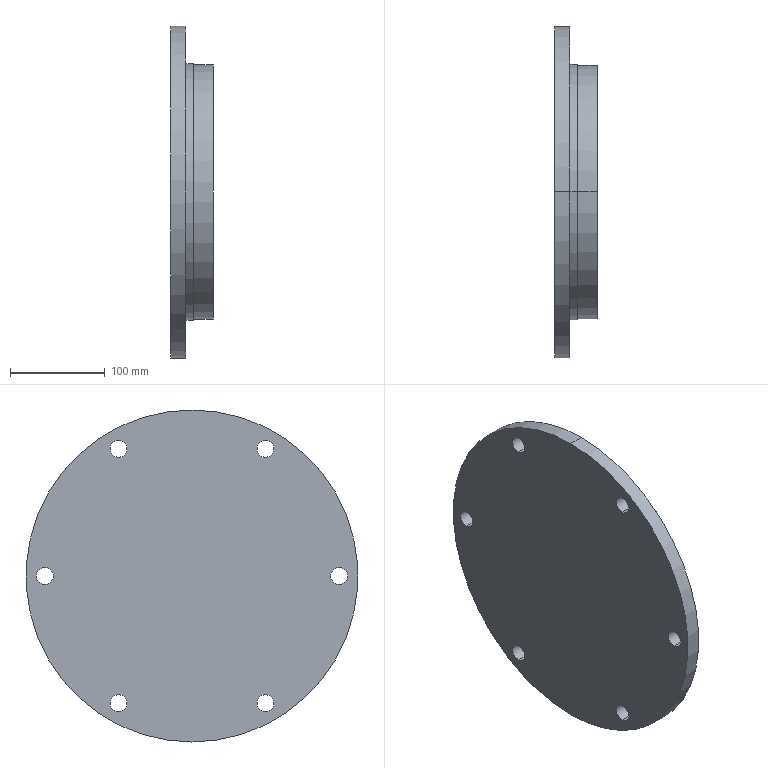Part | NX | features BREP 1 | 1 solid | 27 faces | box 45 x 350 x 350 mm | volume 1642719 mm3 | cylinder 18 | plane 5 | torus 2 | cone 2 | commonest cylinder face diameters 18 x12 268 x2 270 x2 350 x2
STEP:
#1=CARTESIAN_POINT('',(16.,77.5,-143.234));
#2=VERTEX_POINT('',#1);
#3=CARTESIAN_POINT('',(16.,77.5,-125.234));
#4=VERTEX_POINT('',#3);
#5=CARTESIAN_POINT('',(16.,77.5,-134.234));
#6=DIRECTION('',(-1.,0.,0.));
#7=DIRECTION('',(0.,0.,1.));
#8=AXIS2_PLACEMENT_3D('',#5,#6,#7);
#9=CIRCLE('',#8,9.);
#10=EDGE_CURVE('',#2,#4,#9,.T.);
#11=ORIENTED_EDGE('',*,*,#10,.F.);
#12=CARTESIAN_POINT('',(0.,77.5,-143.234));
#13=VERTEX_POINT('',#12);
#14=CARTESIAN_POINT('',(45.,77.5,-143.234));
#15=DIRECTION('',(-1.,0.,0.));
#16=VECTOR('',#15,1000.);
#17=LINE('',#14,#16);
#18=EDGE_CURVE('',#2,#13,#17,.T.);
#19=ORIENTED_EDGE('',*,*,#18,.T.);
#20=CARTESIAN_POINT('',(0.,77.5,-125.234));
#21=VERTEX_POINT('',#20);
#22=CARTESIAN_POINT('',(0.,77.5,-134.234));
#23=DIRECTION('',(-1.,0.,0.));
#24=DIRECTION('',(0.,0.866,0.5));
#25=AXIS2_PLACEMENT_3D('',#22,#23,#24);
#26=CIRCLE('',#25,9.);
#27=EDGE_CURVE('',#13,#21,#26,.T.);
#28=ORIENTED_EDGE('',*,*,#27,.T.);
#29=CARTESIAN_POINT('',(45.,77.5,-125.234));
#30=DIRECTION('',(-1.,0.,0.));
#31=VECTOR('',#30,1000.);
#32=LINE('',#29,#31);
#33=EDGE_CURVE('',#4,#21,#32,.T.);
#34=ORIENTED_EDGE('',*,*,#33,.F.);
#35=EDGE_LOOP('',(#11,#19,#28,#34));
#36=FACE_BOUND('',#35,.T.);
#37=CARTESIAN_POINT('',(45.,77.5,-134.234));
#38=DIRECTION('',(-1.,0.,0.));
#39=DIRECTION('',(0.,0.,-1.));
#40=AXIS2_PLACEMENT_3D('',#37,#38,#39);
#41=CYLINDRICAL_SURFACE('',#40,9.);
#42=ADVANCED_FACE('',(#36),#41,.F.);
#43=CARTESIAN_POINT('',(16.,-77.5,-143.234));
#44=VERTEX_POINT('',#43);
#45=CARTESIAN_POINT('',(16.,-77.5,-125.234));
#46=VERTEX_POINT('',#45);
#47=CARTESIAN_POINT('',(16.,-77.5,-134.234));
#48=DIRECTION('',(-1.,0.,0.));
#49=DIRECTION('',(0.,0.,1.));
#50=AXIS2_PLACEMENT_3D('',#47,#48,#49);
#51=CIRCLE('',#50,9.);
#52=EDGE_CURVE('',#44,#46,#51,.T.);
#53=ORIENTED_EDGE('',*,*,#52,.F.);
#54=CARTESIAN_POINT('',(0.,-77.5,-143.234));
#55=VERTEX_POINT('',#54);
#56=CARTESIAN_POINT('',(45.,-77.5,-143.234));
#57=DIRECTION('',(-1.,0.,0.));
#58=VECTOR('',#57,1000.);
#59=LINE('',#56,#58);
#60=EDGE_CURVE('',#44,#55,#59,.T.);
#61=ORIENTED_EDGE('',*,*,#60,.T.);
#62=CARTESIAN_POINT('',(0.,-77.5,-125.234));
#63=VERTEX_POINT('',#62);
#64=CARTESIAN_POINT('',(0.,-77.5,-134.234));
#65=DIRECTION('',(-1.,0.,0.));
#66=DIRECTION('',(0.,0.866,-0.5));
#67=AXIS2_PLACEMENT_3D('',#64,#65,#66);
#68=CIRCLE('',#67,9.);
#69=EDGE_CURVE('',#55,#63,#68,.T.);
#70=ORIENTED_EDGE('',*,*,#69,.T.);
#71=CARTESIAN_POINT('',(45.,-77.5,-125.234));
#72=DIRECTION('',(-1.,0.,0.));
#73=VECTOR('',#72,1000.);
#74=LINE('',#71,#73);
#75=EDGE_CURVE('',#46,#63,#74,.T.);
#76=ORIENTED_EDGE('',*,*,#75,.F.);
#77=EDGE_LOOP('',(#53,#61,#70,#76));
#78=FACE_BOUND('',#77,.T.);
#79=CARTESIAN_POINT('',(45.,-77.5,-134.234));
#80=DIRECTION('',(-1.,0.,0.));
#81=DIRECTION('',(0.,0.,-1.));
#82=AXIS2_PLACEMENT_3D('',#79,#80,#81);
#83=CYLINDRICAL_SURFACE('',#82,9.);
#84=ADVANCED_FACE('',(#78),#83,.F.);
#85=CARTESIAN_POINT('',(16.,-155.,-9.));
#86=VERTEX_POINT('',#85);
#87=CARTESIAN_POINT('',(16.,-155.,9.));
#88=VERTEX_POINT('',#87);
#89=CARTESIAN_POINT('',(16.,-155.,0.));
#90=DIRECTION('',(-1.,0.,0.));
#91=DIRECTION('',(0.,0.,1.));
#92=AXIS2_PLACEMENT_3D('',#89,#90,#91);
#93=CIRCLE('',#92,9.);
#94=EDGE_CURVE('',#86,#88,#93,.T.);
#95=ORIENTED_EDGE('',*,*,#94,.F.);
#96=CARTESIAN_POINT('',(0.,-155.,-9.));
#97=VERTEX_POINT('',#96);
#98=CARTESIAN_POINT('',(45.,-155.,-9.));
#99=DIRECTION('',(-1.,0.,0.));
#100=VECTOR('',#99,1000.);
#101=LINE('',#98,#100);
#102=EDGE_CURVE('',#86,#97,#101,.T.);
#103=ORIENTED_EDGE('',*,*,#102,.T.);
#104=CARTESIAN_POINT('',(0.,-155.,9.));
#105=VERTEX_POINT('',#104);
#106=CARTESIAN_POINT('',(0.,-155.,0.));
#107=DIRECTION('',(-1.,0.,0.));
#108=DIRECTION('',(0.,0.,-1.));
#109=AXIS2_PLACEMENT_3D('',#106,#107,#108);
#110=CIRCLE('',#109,9.);
#111=EDGE_CURVE('',#97,#105,#110,.T.);
#112=ORIENTED_EDGE('',*,*,#111,.T.);
#113=CARTESIAN_POINT('',(45.,-155.,9.));
#114=DIRECTION('',(-1.,0.,0.));
#115=VECTOR('',#114,1000.);
#116=LINE('',#113,#115);
#117=EDGE_CURVE('',#88,#105,#116,.T.);
#118=ORIENTED_EDGE('',*,*,#117,.F.);
#119=EDGE_LOOP('',(#95,#103,#112,#118));
#120=FACE_BOUND('',#119,.T.);
#121=CARTESIAN_POINT('',(45.,-155.,0.));
#122=DIRECTION('',(-1.,0.,0.));
#123=DIRECTION('',(0.,0.,-1.));
#124=AXIS2_PLACEMENT_3D('',#121,#122,#123);
#125=CYLINDRICAL_SURFACE('',#124,9.);
#126=ADVANCED_FACE('',(#120),#125,.F.);
#127=CARTESIAN_POINT('',(16.,-77.5,125.234));
#128=VERTEX_POINT('',#127);
#129=CARTESIAN_POINT('',(16.,-77.5,143.234));
#130=VERTEX_POINT('',#129);
#131=CARTESIAN_POINT('',(16.,-77.5,134.234));
#132=DIRECTION('',(-1.,0.,0.));
#133=DIRECTION('',(0.,0.,1.));
#134=AXIS2_PLACEMENT_3D('',#131,#132,#133);
#135=CIRCLE('',#134,9.);
#136=EDGE_CURVE('',#128,#130,#135,.T.);
#137=ORIENTED_EDGE('',*,*,#136,.F.);
#138=CARTESIAN_POINT('',(0.,-77.5,125.234));
#139=VERTEX_POINT('',#138);
#140=CARTESIAN_POINT('',(45.,-77.5,125.234));
#141=DIRECTION('',(-1.,0.,0.));
#142=VECTOR('',#141,1000.);
#143=LINE('',#140,#142);
#144=EDGE_CURVE('',#128,#139,#143,.T.);
#145=ORIENTED_EDGE('',*,*,#144,.T.);
#146=CARTESIAN_POINT('',(0.,-77.5,143.234));
#147=VERTEX_POINT('',#146);
#148=CARTESIAN_POINT('',(0.,-77.5,134.234));
#149=DIRECTION('',(-1.,0.,0.));
#150=DIRECTION('',(0.,-0.866,-0.5));
#151=AXIS2_PLACEMENT_3D('',#148,#149,#150);
#152=CIRCLE('',#151,9.);
#153=EDGE_CURVE('',#139,#147,#152,.T.);
#154=ORIENTED_EDGE('',*,*,#153,.T.);
#155=CARTESIAN_POINT('',(45.,-77.5,143.234));
#156=DIRECTION('',(-1.,0.,0.));
#157=VECTOR('',#156,1000.);
#158=LINE('',#155,#157);
#159=EDGE_CURVE('',#130,#147,#158,.T.);
#160=ORIENTED_EDGE('',*,*,#159,.F.);
#161=EDGE_LOOP('',(#137,#145,#154,#160));
#162=FACE_BOUND('',#161,.T.);
#163=CARTESIAN_POINT('',(45.,-77.5,134.234));
#164=DIRECTION('',(-1.,0.,0.));
#165=DIRECTION('',(0.,0.,-1.));
#166=AXIS2_PLACEMENT_3D('',#163,#164,#165);
#167=CYLINDRICAL_SURFACE('',#166,9.);
#168=ADVANCED_FACE('',(#162),#167,.F.);
#169=CARTESIAN_POINT('',(16.,77.5,125.234));
#170=VERTEX_POINT('',#169);
#171=CARTESIAN_POINT('',(16.,77.5,143.234));
#172=VERTEX_POINT('',#171);
#173=CARTESIAN_POINT('',(16.,77.5,134.234));
#174=DIRECTION('',(-1.,0.,0.));
#175=DIRECTION('',(0.,0.,1.));
#176=AXIS2_PLACEMENT_3D('',#173,#174,#175);
#177=CIRCLE('',#176,9.);
#178=EDGE_CURVE('',#170,#172,#177,.T.);
#179=ORIENTED_EDGE('',*,*,#178,.F.);
#180=CARTESIAN_POINT('',(0.,77.5,125.234));
#181=VERTEX_POINT('',#180);
#182=CARTESIAN_POINT('',(45.,77.5,125.234));
#183=DIRECTION('',(-1.,0.,0.));
#184=VECTOR('',#183,1000.);
#185=LINE('',#182,#184);
#186=EDGE_CURVE('',#170,#181,#185,.T.);
#187=ORIENTED_EDGE('',*,*,#186,.T.);
#188=CARTESIAN_POINT('',(0.,77.5,143.234));
#189=VERTEX_POINT('',#188);
#190=CARTESIAN_POINT('',(0.,77.5,134.234));
#191=DIRECTION('',(-1.,0.,0.));
#192=DIRECTION('',(0.,-0.866,0.5));
#193=AXIS2_PLACEMENT_3D('',#190,#191,#192);
#194=CIRCLE('',#193,9.);
#195=EDGE_CURVE('',#181,#189,#194,.T.);
#196=ORIENTED_EDGE('',*,*,#195,.T.);
#197=CARTESIAN_POINT('',(45.,77.5,143.234));
#198=DIRECTION('',(-1.,0.,0.));
#199=VECTOR('',#198,1000.);
#200=LINE('',#197,#199);
#201=EDGE_CURVE('',#172,#189,#200,.T.);
#202=ORIENTED_EDGE('',*,*,#201,.F.);
#203=EDGE_LOOP('',(#179,#187,#196,#202));
#204=FACE_BOUND('',#203,.T.);
#205=CARTESIAN_POINT('',(45.,77.5,134.234));
#206=DIRECTION('',(-1.,0.,0.));
#207=DIRECTION('',(0.,0.,-1.));
#208=AXIS2_PLACEMENT_3D('',#205,#206,#207);
#209=CYLINDRICAL_SURFACE('',#208,9.);
#210=ADVANCED_FACE('',(#204),#209,.F.);
#211=CARTESIAN_POINT('',(16.,155.,-9.));
#212=VERTEX_POINT('',#211);
#213=CARTESIAN_POINT('',(16.,155.,9.));
#214=VERTEX_POINT('',#213);
#215=CARTESIAN_POINT('',(16.,155.,0.));
#216=DIRECTION('',(-1.,0.,0.));
#217=DIRECTION('',(0.,0.,1.));
#218=AXIS2_PLACEMENT_3D('',#215,#216,#217);
#219=CIRCLE('',#218,9.);
#220=EDGE_CURVE('',#212,#214,#219,.T.);
#221=ORIENTED_EDGE('',*,*,#220,.F.);
#222=CARTESIAN_POINT('',(0.,155.,-9.));
#223=VERTEX_POINT('',#222);
#224=CARTESIAN_POINT('',(45.,155.,-9.));
#225=DIRECTION('',(-1.,0.,0.));
#226=VECTOR('',#225,1000.);
#227=LINE('',#224,#226);
#228=EDGE_CURVE('',#212,#223,#227,.T.);
#229=ORIENTED_EDGE('',*,*,#228,.T.);
#230=CARTESIAN_POINT('',(0.,155.,9.));
#231=VERTEX_POINT('',#230);
#232=CARTESIAN_POINT('',(0.,155.,0.));
#233=DIRECTION('',(-1.,0.,0.));
#234=DIRECTION('',(0.,0.,1.));
#235=AXIS2_PLACEMENT_3D('',#232,#233,#234);
#236=CIRCLE('',#235,9.);
#237=EDGE_CURVE('',#223,#231,#236,.T.);
#238=ORIENTED_EDGE('',*,*,#237,.T.);
#239=CARTESIAN_POINT('',(45.,155.,9.));
#240=DIRECTION('',(-1.,0.,0.));
#241=VECTOR('',#240,1000.);
#242=LINE('',#239,#241);
#243=EDGE_CURVE('',#214,#231,#242,.T.);
#244=ORIENTED_EDGE('',*,*,#243,.F.);
#245=EDGE_LOOP('',(#221,#229,#238,#244));
#246=FACE_BOUND('',#245,.T.);
#247=CARTESIAN_POINT('',(45.,155.,0.));
#248=DIRECTION('',(-1.,0.,0.));
#249=DIRECTION('',(0.,0.,-1.));
#250=AXIS2_PLACEMENT_3D('',#247,#248,#249);
#251=CYLINDRICAL_SURFACE('',#250,9.);
#252=ADVANCED_FACE('',(#246),#251,.F.);
#253=CARTESIAN_POINT('',(16.061,0.,-112.597));
#254=VERTEX_POINT('',#253);
#255=CARTESIAN_POINT('',(16.061,0.,112.597));
#256=VERTEX_POINT('',#255);
#257=CARTESIAN_POINT('',(16.061,0.,0.));
#258=DIRECTION('',(-1.,0.,0.));
#259=DIRECTION('',(0.,0.,1.));
#260=AXIS2_PLACEMENT_3D('',#257,#258,#259);
#261=CIRCLE('',#260,112.597);
#262=EDGE_CURVE('',#254,#256,#261,.T.);
#263=ORIENTED_EDGE('',*,*,#262,.F.);
#264=CARTESIAN_POINT('',(10.,0.,-103.406));
#265=VERTEX_POINT('',#264);
#266=CARTESIAN_POINT('',(20.,0.,-103.406));
#267=DIRECTION('',(0.,1.,0.));
#268=DIRECTION('',(0.,0.,1.));
#269=AXIS2_PLACEMENT_3D('',#266,#267,#268);
#270=CIRCLE('',#269,10.);
#271=EDGE_CURVE('',#254,#265,#270,.T.);
#272=ORIENTED_EDGE('',*,*,#271,.T.);
#273=CARTESIAN_POINT('',(10.,0.,103.406));
#274=VERTEX_POINT('',#273);
#275=CARTESIAN_POINT('',(10.,0.,0.));
#276=DIRECTION('',(-1.,0.,0.));
#277=DIRECTION('',(0.,0.,1.));
#278=AXIS2_PLACEMENT_3D('',#275,#276,#277);
#279=CIRCLE('',#278,103.406);
#280=EDGE_CURVE('',#265,#274,#279,.T.);
#281=ORIENTED_EDGE('',*,*,#280,.T.);
#282=CARTESIAN_POINT('',(20.,0.,103.406));
#283=DIRECTION('',(0.,-1.,0.));
#284=DIRECTION('',(0.,0.,-1.));
#285=AXIS2_PLACEMENT_3D('',#282,#283,#284);
#286=CIRCLE('',#285,10.);
#287=EDGE_CURVE('',#256,#274,#286,.T.);
#288=ORIENTED_EDGE('',*,*,#287,.F.);
#289=EDGE_LOOP('',(#263,#272,#281,#288));
#290=FACE_BOUND('',#289,.T.);
#291=CARTESIAN_POINT('',(20.,0.,0.));
#292=DIRECTION('',(-1.,0.,0.));
#293=DIRECTION('',(0.,0.,-1.));
#294=AXIS2_PLACEMENT_3D('',#291,#292,#293);
#295=TOROIDAL_SURFACE('',#294,103.406,10.);
#296=ADVANCED_FACE('',(#290),#295,.F.);
#297=ORIENTED_EDGE('',*,*,#262,.T.);
#298=CARTESIAN_POINT('',(45.,0.,125.));
#299=VERTEX_POINT('',#298);
#300=CARTESIAN_POINT('',(16.061,0.,112.597));
#301=DIRECTION('',(0.9191,0.,0.3939));
#302=VECTOR('',#301,1000.);
#303=LINE('',#300,#302);
#304=EDGE_CURVE('',#299,#256,#303,.F.);
#305=ORIENTED_EDGE('',*,*,#304,.F.);
#306=CARTESIAN_POINT('',(45.,0.,-125.));
#307=VERTEX_POINT('',#306);
#308=CARTESIAN_POINT('',(45.,0.,0.));
#309=DIRECTION('',(-1.,0.,0.));
#310=DIRECTION('',(0.,0.,1.));
#311=AXIS2_PLACEMENT_3D('',#308,#309,#310);
#312=CIRCLE('',#311,125.);
#313=EDGE_CURVE('',#307,#299,#312,.T.);
#314=ORIENTED_EDGE('',*,*,#313,.F.);
#315=CARTESIAN_POINT('',(16.061,0.,-112.597));
#316=DIRECTION('',(0.9191,0.,-0.3939));
#317=VECTOR('',#316,1000.);
#318=LINE('',#315,#317);
#319=EDGE_CURVE('',#307,#254,#318,.F.);
#320=ORIENTED_EDGE('',*,*,#319,.T.);
#321=EDGE_LOOP('',(#297,#305,#314,#320));
#322=FACE_BOUND('',#321,.T.);
#323=CARTESIAN_POINT('',(16.061,0.,0.));
#324=DIRECTION('',(1.,0.,0.));
#325=DIRECTION('',(0.,0.,1.));
#326=AXIS2_PLACEMENT_3D('',#323,#324,#325);
#327=CONICAL_SURFACE('',#326,112.597,0.4049);
#328=ADVANCED_FACE('',(#322),#327,.F.);
#329=CARTESIAN_POINT('',(45.,0.,134.));
#330=VERTEX_POINT('',#329);
#331=CARTESIAN_POINT('',(45.,0.,-134.));
#332=VERTEX_POINT('',#331);
#333=CARTESIAN_POINT('',(45.,0.,0.));
#334=DIRECTION('',(-1.,0.,0.));
#335=DIRECTION('',(0.,0.,1.));
#336=AXIS2_PLACEMENT_3D('',#333,#334,#335);
#337=CIRCLE('',#336,134.);
#338=EDGE_CURVE('',#330,#332,#337,.T.);
#339=ORIENTED_EDGE('',*,*,#338,.T.);
#340=CARTESIAN_POINT('',(24.,0.,-134.));
#341=VERTEX_POINT('',#340);
#342=CARTESIAN_POINT('',(0.,0.,-134.));
#343=DIRECTION('',(-1.,0.,0.));
#344=VECTOR('',#343,1000.);
#345=LINE('',#342,#344);
#346=EDGE_CURVE('',#332,#341,#345,.T.);
#347=ORIENTED_EDGE('',*,*,#346,.T.);
#348=CARTESIAN_POINT('',(24.,0.,134.));
#349=VERTEX_POINT('',#348);
#350=CARTESIAN_POINT('',(24.,0.,0.));
#351=DIRECTION('',(-1.,0.,0.));
#352=DIRECTION('',(0.,0.,1.));
#353=AXIS2_PLACEMENT_3D('',#350,#351,#352);
#354=CIRCLE('',#353,134.);
#355=EDGE_CURVE('',#349,#341,#354,.T.);
#356=ORIENTED_EDGE('',*,*,#355,.F.);
#357=CARTESIAN_POINT('',(0.,0.,134.));
#358=DIRECTION('',(-1.,0.,0.));
#359=VECTOR('',#358,1000.);
#360=LINE('',#357,#359);
#361=EDGE_CURVE('',#330,#349,#360,.T.);
#362=ORIENTED_EDGE('',*,*,#361,.F.);
#363=EDGE_LOOP('',(#339,#347,#356,#362));
#364=FACE_BOUND('',#363,.T.);
#365=CARTESIAN_POINT('',(0.,0.,0.));
#366=DIRECTION('',(-1.,0.,0.));
#367=DIRECTION('',(0.,0.,-1.));
#368=AXIS2_PLACEMENT_3D('',#365,#366,#367);
#369=CYLINDRICAL_SURFACE('',#368,134.);
#370=ADVANCED_FACE('',(#364),#369,.T.);
#371=CARTESIAN_POINT('',(24.,0.,135.));
#372=VERTEX_POINT('',#371);
#373=CARTESIAN_POINT('',(24.,0.,-135.));
#374=VERTEX_POINT('',#373);
#375=CARTESIAN_POINT('',(24.,0.,0.));
#376=DIRECTION('',(-1.,0.,0.));
#377=DIRECTION('',(0.,0.,1.));
#378=AXIS2_PLACEMENT_3D('',#375,#376,#377);
#379=CIRCLE('',#378,135.);
#380=EDGE_CURVE('',#372,#374,#379,.T.);
#381=ORIENTED_EDGE('',*,*,#380,.T.);
#382=CARTESIAN_POINT('',(16.,0.,-135.));
#383=VERTEX_POINT('',#382);
#384=CARTESIAN_POINT('',(0.,0.,-135.));
#385=DIRECTION('',(-1.,0.,0.));
#386=VECTOR('',#385,1000.);
#387=LINE('',#384,#386);
#388=EDGE_CURVE('',#374,#383,#387,.T.);
#389=ORIENTED_EDGE('',*,*,#388,.T.);
#390=CARTESIAN_POINT('',(16.,0.,135.));
#391=VERTEX_POINT('',#390);
#392=CARTESIAN_POINT('',(16.,0.,0.));
#393=DIRECTION('',(-1.,0.,0.));
#394=DIRECTION('',(0.,0.,1.));
#395=AXIS2_PLACEMENT_3D('',#392,#393,#394);
#396=CIRCLE('',#395,135.);
#397=EDGE_CURVE('',#391,#383,#396,.T.);
#398=ORIENTED_EDGE('',*,*,#397,.F.);
#399=CARTESIAN_POINT('',(0.,0.,135.));
#400=DIRECTION('',(-1.,0.,0.));
#401=VECTOR('',#400,1000.);
#402=LINE('',#399,#401);
#403=EDGE_CURVE('',#372,#391,#402,.T.);
#404=ORIENTED_EDGE('',*,*,#403,.F.);
#405=EDGE_LOOP('',(#381,#389,#398,#404));
#406=FACE_BOUND('',#405,.T.);
#407=CARTESIAN_POINT('',(0.,0.,0.));
#408=DIRECTION('',(-1.,0.,0.));
#409=DIRECTION('',(0.,0.,-1.));
#410=AXIS2_PLACEMENT_3D('',#407,#408,#409);
#411=CYLINDRICAL_SURFACE('',#410,135.);
#412=ADVANCED_FACE('',(#406),#411,.T.);
#413=CARTESIAN_POINT('',(16.,0.,175.));
#414=VERTEX_POINT('',#413);
#415=CARTESIAN_POINT('',(16.,0.,-175.));
#416=VERTEX_POINT('',#415);
#417=CARTESIAN_POINT('',(16.,0.,0.));
#418=DIRECTION('',(-1.,0.,0.));
#419=DIRECTION('',(0.,0.,1.));
#420=AXIS2_PLACEMENT_3D('',#417,#418,#419);
#421=CIRCLE('',#420,175.);
#422=EDGE_CURVE('',#414,#416,#421,.T.);
#423=ORIENTED_EDGE('',*,*,#422,.T.);
#424=CARTESIAN_POINT('',(0.,0.,-175.));
#425=VERTEX_POINT('',#424);
#426=CARTESIAN_POINT('',(0.,0.,-175.));
#427=DIRECTION('',(-1.,0.,0.));
#428=VECTOR('',#427,1000.);
#429=LINE('',#426,#428);
#430=EDGE_CURVE('',#416,#425,#429,.T.);
#431=ORIENTED_EDGE('',*,*,#430,.T.);
#432=CARTESIAN_POINT('',(0.,0.,175.));
#433=VERTEX_POINT('',#432);
#434=CARTESIAN_POINT('',(0.,0.,0.));
#435=DIRECTION('',(-1.,0.,0.));
#436=DIRECTION('',(0.,0.,1.));
#437=AXIS2_PLACEMENT_3D('',#434,#435,#436);
#438=CIRCLE('',#437,175.);
#439=EDGE_CURVE('',#433,#425,#438,.T.);
#440=ORIENTED_EDGE('',*,*,#439,.F.);
#441=CARTESIAN_POINT('',(0.,0.,175.));
#442=DIRECTION('',(-1.,0.,0.));
#443=VECTOR('',#442,1000.);
#444=LINE('',#441,#443);
#445=EDGE_CURVE('',#414,#433,#444,.T.);
#446=ORIENTED_EDGE('',*,*,#445,.F.);
#447=EDGE_LOOP('',(#423,#431,#440,#446));
#448=FACE_BOUND('',#447,.T.);
#449=CARTESIAN_POINT('',(0.,0.,0.));
#450=DIRECTION('',(-1.,0.,0.));
#451=DIRECTION('',(0.,0.,-1.));
#452=AXIS2_PLACEMENT_3D('',#449,#450,#451);
#453=CYLINDRICAL_SURFACE('',#452,175.);
#454=ADVANCED_FACE('',(#448),#453,.T.);
#455=CARTESIAN_POINT('',(0.,77.5,-134.234));
#456=DIRECTION('',(-1.,0.,0.));
#457=DIRECTION('',(0.,0.866,0.5));
#458=AXIS2_PLACEMENT_3D('',#455,#456,#457);
#459=CIRCLE('',#458,9.);
#460=EDGE_CURVE('',#21,#13,#459,.T.);
#461=ORIENTED_EDGE('',*,*,#460,.F.);
#462=ORIENTED_EDGE('',*,*,#27,.F.);
#463=EDGE_LOOP('',(#461,#462));
#464=FACE_BOUND('',#463,.T.);
#465=CARTESIAN_POINT('',(0.,-77.5,-134.234));
#466=DIRECTION('',(-1.,0.,0.));
#467=DIRECTION('',(0.,0.866,-0.5));
#468=AXIS2_PLACEMENT_3D('',#465,#466,#467);
#469=CIRCLE('',#468,9.);
#470=EDGE_CURVE('',#63,#55,#469,.T.);
#471=ORIENTED_EDGE('',*,*,#470,.F.);
#472=ORIENTED_EDGE('',*,*,#69,.F.);
#473=EDGE_LOOP('',(#471,#472));
#474=FACE_BOUND('',#473,.T.);
#475=CARTESIAN_POINT('',(0.,-155.,0.));
#476=DIRECTION('',(-1.,0.,0.));
#477=DIRECTION('',(0.,0.,-1.));
#478=AXIS2_PLACEMENT_3D('',#475,#476,#477);
#479=CIRCLE('',#478,9.);
#480=EDGE_CURVE('',#105,#97,#479,.T.);
#481=ORIENTED_EDGE('',*,*,#480,.F.);
#482=ORIENTED_EDGE('',*,*,#111,.F.);
#483=EDGE_LOOP('',(#481,#482));
#484=FACE_BOUND('',#483,.T.);
#485=CARTESIAN_POINT('',(0.,-77.5,134.234));
#486=DIRECTION('',(-1.,0.,0.));
#487=DIRECTION('',(0.,-0.866,-0.5));
#488=AXIS2_PLACEMENT_3D('',#485,#486,#487);
#489=CIRCLE('',#488,9.);
#490=EDGE_CURVE('',#147,#139,#489,.T.);
#491=ORIENTED_EDGE('',*,*,#490,.F.);
#492=ORIENTED_EDGE('',*,*,#153,.F.);
#493=EDGE_LOOP('',(#491,#492));
#494=FACE_BOUND('',#493,.T.);
#495=CARTESIAN_POINT('',(0.,77.5,134.234));
#496=DIRECTION('',(-1.,0.,0.));
#497=DIRECTION('',(0.,-0.866,0.5));
#498=AXIS2_PLACEMENT_3D('',#495,#496,#497);
#499=CIRCLE('',#498,9.);
#500=EDGE_CURVE('',#189,#181,#499,.T.);
#501=ORIENTED_EDGE('',*,*,#500,.F.);
#502=ORIENTED_EDGE('',*,*,#195,.F.);
#503=EDGE_LOOP('',(#501,#502));
#504=FACE_BOUND('',#503,.T.);
#505=CARTESIAN_POINT('',(0.,155.,0.));
#506=DIRECTION('',(-1.,0.,0.));
#507=DIRECTION('',(0.,0.,1.));
#508=AXIS2_PLACEMENT_3D('',#505,#506,#507);
#509=CIRCLE('',#508,9.);
#510=EDGE_CURVE('',#231,#223,#509,.T.);
#511=ORIENTED_EDGE('',*,*,#510,.F.);
#512=ORIENTED_EDGE('',*,*,#237,.F.);
#513=EDGE_LOOP('',(#511,#512));
#514=FACE_BOUND('',#513,.T.);
#515=ORIENTED_EDGE('',*,*,#439,.T.);
#516=CARTESIAN_POINT('',(0.,0.,0.));
#517=DIRECTION('',(-1.,0.,0.));
#518=DIRECTION('',(0.,0.,1.));
#519=AXIS2_PLACEMENT_3D('',#516,#517,#518);
#520=CIRCLE('',#519,175.);
#521=EDGE_CURVE('',#425,#433,#520,.T.);
#522=ORIENTED_EDGE('',*,*,#521,.T.);
#523=EDGE_LOOP('',(#515,#522));
#524=FACE_BOUND('',#523,.T.);
#525=CARTESIAN_POINT('',(0.,0.,0.));
#526=DIRECTION('',(1.,0.,0.));
#527=DIRECTION('',(0.,0.,1.));
#528=AXIS2_PLACEMENT_3D('',#525,#526,#527);
#529=PLANE('',#528);
#530=ADVANCED_FACE('',(#464,#474,#484,#494,#504,#514,#524),#529,.F.);
#531=ORIENTED_EDGE('',*,*,#430,.F.);
#532=CARTESIAN_POINT('',(16.,0.,0.));
#533=DIRECTION('',(-1.,0.,0.));
#534=DIRECTION('',(0.,0.,1.));
#535=AXIS2_PLACEMENT_3D('',#532,#533,#534);
#536=CIRCLE('',#535,175.);
#537=EDGE_CURVE('',#416,#414,#536,.T.);
#538=ORIENTED_EDGE('',*,*,#537,.T.);
#539=ORIENTED_EDGE('',*,*,#445,.T.);
#540=ORIENTED_EDGE('',*,*,#521,.F.);
#541=EDGE_LOOP('',(#531,#538,#539,#540));
#542=FACE_BOUND('',#541,.T.);
#543=CARTESIAN_POINT('',(0.,0.,0.));
#544=DIRECTION('',(-1.,0.,0.));
#545=DIRECTION('',(0.,0.,-1.));
#546=AXIS2_PLACEMENT_3D('',#543,#544,#545);
#547=CYLINDRICAL_SURFACE('',#546,175.);
#548=ADVANCED_FACE('',(#542),#547,.T.);
#549=CARTESIAN_POINT('',(16.,77.5,-134.234));
#550=DIRECTION('',(-1.,0.,0.));
#551=DIRECTION('',(0.,0.,1.));
#552=AXIS2_PLACEMENT_3D('',#549,#550,#551);
#553=CIRCLE('',#552,9.);
#554=EDGE_CURVE('',#4,#2,#553,.T.);
#555=ORIENTED_EDGE('',*,*,#554,.T.);
#556=ORIENTED_EDGE('',*,*,#10,.T.);
#557=EDGE_LOOP('',(#555,#556));
#558=FACE_BOUND('',#557,.T.);
#559=CARTESIAN_POINT('',(16.,-77.5,-134.234));
#560=DIRECTION('',(-1.,0.,0.));
#561=DIRECTION('',(0.,0.,1.));
#562=AXIS2_PLACEMENT_3D('',#559,#560,#561);
#563=CIRCLE('',#562,9.);
#564=EDGE_CURVE('',#46,#44,#563,.T.);
#565=ORIENTED_EDGE('',*,*,#564,.T.);
#566=ORIENTED_EDGE('',*,*,#52,.T.);
#567=EDGE_LOOP('',(#565,#566));
#568=FACE_BOUND('',#567,.T.);
#569=CARTESIAN_POINT('',(16.,-155.,0.));
#570=DIRECTION('',(-1.,0.,0.));
#571=DIRECTION('',(0.,0.,1.));
#572=AXIS2_PLACEMENT_3D('',#569,#570,#571);
#573=CIRCLE('',#572,9.);
#574=EDGE_CURVE('',#88,#86,#573,.T.);
#575=ORIENTED_EDGE('',*,*,#574,.T.);
#576=ORIENTED_EDGE('',*,*,#94,.T.);
#577=EDGE_LOOP('',(#575,#576));
#578=FACE_BOUND('',#577,.T.);
#579=CARTESIAN_POINT('',(16.,-77.5,134.234));
#580=DIRECTION('',(-1.,0.,0.));
#581=DIRECTION('',(0.,0.,1.));
#582=AXIS2_PLACEMENT_3D('',#579,#580,#581);
#583=CIRCLE('',#582,9.);
#584=EDGE_CURVE('',#130,#128,#583,.T.);
#585=ORIENTED_EDGE('',*,*,#584,.T.);
#586=ORIENTED_EDGE('',*,*,#136,.T.);
#587=EDGE_LOOP('',(#585,#586));
#588=FACE_BOUND('',#587,.T.);
#589=CARTESIAN_POINT('',(16.,77.5,134.234));
#590=DIRECTION('',(-1.,0.,0.));
#591=DIRECTION('',(0.,0.,1.));
#592=AXIS2_PLACEMENT_3D('',#589,#590,#591);
#593=CIRCLE('',#592,9.);
#594=EDGE_CURVE('',#172,#170,#593,.T.);
#595=ORIENTED_EDGE('',*,*,#594,.T.);
#596=ORIENTED_EDGE('',*,*,#178,.T.);
#597=EDGE_LOOP('',(#595,#596));
#598=FACE_BOUND('',#597,.T.);
#599=CARTESIAN_POINT('',(16.,155.,0.));
#600=DIRECTION('',(-1.,0.,0.));
#601=DIRECTION('',(0.,0.,1.));
#602=AXIS2_PLACEMENT_3D('',#599,#600,#601);
#603=CIRCLE('',#602,9.);
#604=EDGE_CURVE('',#214,#212,#603,.T.);
#605=ORIENTED_EDGE('',*,*,#604,.T.);
#606=ORIENTED_EDGE('',*,*,#220,.T.);
#607=EDGE_LOOP('',(#605,#606));
#608=FACE_BOUND('',#607,.T.);
#609=ORIENTED_EDGE('',*,*,#422,.F.);
#610=ORIENTED_EDGE('',*,*,#537,.F.);
#611=EDGE_LOOP('',(#609,#610));
#612=FACE_BOUND('',#611,.T.);
#613=ORIENTED_EDGE('',*,*,#397,.T.);
#614=CARTESIAN_POINT('',(16.,0.,0.));
#615=DIRECTION('',(-1.,0.,0.));
#616=DIRECTION('',(0.,0.,1.));
#617=AXIS2_PLACEMENT_3D('',#614,#615,#616);
#618=CIRCLE('',#617,135.);
#619=EDGE_CURVE('',#383,#391,#618,.T.);
#620=ORIENTED_EDGE('',*,*,#619,.T.);
#621=EDGE_LOOP('',(#613,#620));
#622=FACE_BOUND('',#621,.T.);
#623=CARTESIAN_POINT('',(16.,175.,0.));
#624=DIRECTION('',(-1.,0.,0.));
#625=DIRECTION('',(0.,0.,-1.));
#626=AXIS2_PLACEMENT_3D('',#623,#624,#625);
#627=PLANE('',#626);
#628=ADVANCED_FACE('',(#558,#568,#578,#588,#598,#608,#612,#622),#627,.F.);
#629=ORIENTED_EDGE('',*,*,#388,.F.);
#630=CARTESIAN_POINT('',(24.,0.,0.));
#631=DIRECTION('',(-1.,0.,0.));
#632=DIRECTION('',(0.,0.,1.));
#633=AXIS2_PLACEMENT_3D('',#630,#631,#632);
#634=CIRCLE('',#633,135.);
#635=EDGE_CURVE('',#374,#372,#634,.T.);
#636=ORIENTED_EDGE('',*,*,#635,.T.);
#637=ORIENTED_EDGE('',*,*,#403,.T.);
#638=ORIENTED_EDGE('',*,*,#619,.F.);
#639=EDGE_LOOP('',(#629,#636,#637,#638));
#640=FACE_BOUND('',#639,.T.);
#641=CARTESIAN_POINT('',(0.,0.,0.));
#642=DIRECTION('',(-1.,0.,0.));
#643=DIRECTION('',(0.,0.,-1.));
#644=AXIS2_PLACEMENT_3D('',#641,#642,#643);
#645=CYLINDRICAL_SURFACE('',#644,135.);
#646=ADVANCED_FACE('',(#640),#645,.T.);
#647=ORIENTED_EDGE('',*,*,#380,.F.);
#648=ORIENTED_EDGE('',*,*,#635,.F.);
#649=EDGE_LOOP('',(#647,#648));
#650=FACE_BOUND('',#649,.T.);
#651=ORIENTED_EDGE('',*,*,#355,.T.);
#652=CARTESIAN_POINT('',(24.,0.,0.));
#653=DIRECTION('',(-1.,0.,0.));
#654=DIRECTION('',(0.,0.,1.));
#655=AXIS2_PLACEMENT_3D('',#652,#653,#654);
#656=CIRCLE('',#655,134.);
#657=EDGE_CURVE('',#341,#349,#656,.T.);
#658=ORIENTED_EDGE('',*,*,#657,.T.);
#659=EDGE_LOOP('',(#651,#658));
#660=FACE_BOUND('',#659,.T.);
#661=CARTESIAN_POINT('',(24.,135.,0.));
#662=DIRECTION('',(-1.,0.,0.));
#663=DIRECTION('',(0.,0.,-1.));
#664=AXIS2_PLACEMENT_3D('',#661,#662,#663);
#665=PLANE('',#664);
#666=ADVANCED_FACE('',(#650,#660),#665,.F.);
#667=ORIENTED_EDGE('',*,*,#346,.F.);
#668=CARTESIAN_POINT('',(45.,0.,0.));
#669=DIRECTION('',(-1.,0.,0.));
#670=DIRECTION('',(0.,0.,1.));
#671=AXIS2_PLACEMENT_3D('',#668,#669,#670);
#672=CIRCLE('',#671,134.);
#673=EDGE_CURVE('',#332,#330,#672,.T.);
#674=ORIENTED_EDGE('',*,*,#673,.T.);
#675=ORIENTED_EDGE('',*,*,#361,.T.);
#676=ORIENTED_EDGE('',*,*,#657,.F.);
#677=EDGE_LOOP('',(#667,#674,#675,#676));
#678=FACE_BOUND('',#677,.T.);
#679=CARTESIAN_POINT('',(0.,0.,0.));
#680=DIRECTION('',(-1.,0.,0.));
#681=DIRECTION('',(0.,0.,-1.));
#682=AXIS2_PLACEMENT_3D('',#679,#680,#681);
#683=CYLINDRICAL_SURFACE('',#682,134.);
#684=ADVANCED_FACE('',(#678),#683,.T.);
#685=ORIENTED_EDGE('',*,*,#338,.F.);
#686=ORIENTED_EDGE('',*,*,#673,.F.);
#687=EDGE_LOOP('',(#685,#686));
#688=FACE_BOUND('',#687,.T.);
#689=ORIENTED_EDGE('',*,*,#313,.T.);
#690=CARTESIAN_POINT('',(45.,0.,0.));
#691=DIRECTION('',(-1.,0.,0.));
#692=DIRECTION('',(0.,0.,1.));
#693=AXIS2_PLACEMENT_3D('',#690,#691,#692);
#694=CIRCLE('',#693,125.);
#695=EDGE_CURVE('',#299,#307,#694,.T.);
#696=ORIENTED_EDGE('',*,*,#695,.T.);
#697=EDGE_LOOP('',(#689,#696));
#698=FACE_BOUND('',#697,.T.);
#699=CARTESIAN_POINT('',(45.,134.,0.));
#700=DIRECTION('',(-1.,0.,0.));
#701=DIRECTION('',(0.,0.,-1.));
#702=AXIS2_PLACEMENT_3D('',#699,#700,#701);
#703=PLANE('',#702);
#704=ADVANCED_FACE('',(#688,#698),#703,.F.);
#705=ORIENTED_EDGE('',*,*,#304,.T.);
#706=CARTESIAN_POINT('',(16.061,0.,0.));
#707=DIRECTION('',(-1.,0.,0.));
#708=DIRECTION('',(0.,0.,1.));
#709=AXIS2_PLACEMENT_3D('',#706,#707,#708);
#710=CIRCLE('',#709,112.597);
#711=EDGE_CURVE('',#256,#254,#710,.T.);
#712=ORIENTED_EDGE('',*,*,#711,.T.);
#713=ORIENTED_EDGE('',*,*,#319,.F.);
#714=ORIENTED_EDGE('',*,*,#695,.F.);
#715=EDGE_LOOP('',(#705,#712,#713,#714));
#716=FACE_BOUND('',#715,.T.);
#717=CARTESIAN_POINT('',(16.061,0.,0.));
#718=DIRECTION('',(1.,0.,0.));
#719=DIRECTION('',(0.,0.,1.));
#720=AXIS2_PLACEMENT_3D('',#717,#718,#719);
#721=CONICAL_SURFACE('',#720,112.597,0.4049);
#722=ADVANCED_FACE('',(#716),#721,.F.);
#723=ORIENTED_EDGE('',*,*,#271,.F.);
#724=ORIENTED_EDGE('',*,*,#711,.F.);
#725=ORIENTED_EDGE('',*,*,#287,.T.);
#726=CARTESIAN_POINT('',(10.,0.,0.));
#727=DIRECTION('',(-1.,0.,0.));
#728=DIRECTION('',(0.,0.,1.));
#729=AXIS2_PLACEMENT_3D('',#726,#727,#728);
#730=CIRCLE('',#729,103.406);
#731=EDGE_CURVE('',#274,#265,#730,.T.);
#732=ORIENTED_EDGE('',*,*,#731,.T.);
#733=EDGE_LOOP('',(#723,#724,#725,#732));
#734=FACE_BOUND('',#733,.T.);
#735=CARTESIAN_POINT('',(20.,0.,0.));
#736=DIRECTION('',(-1.,0.,0.));
#737=DIRECTION('',(0.,0.,-1.));
#738=AXIS2_PLACEMENT_3D('',#735,#736,#737);
#739=TOROIDAL_SURFACE('',#738,103.406,10.);
#740=ADVANCED_FACE('',(#734),#739,.F.);
#741=ORIENTED_EDGE('',*,*,#731,.F.);
#742=ORIENTED_EDGE('',*,*,#280,.F.);
#743=EDGE_LOOP('',(#741,#742));
#744=FACE_BOUND('',#743,.T.);
#745=CARTESIAN_POINT('',(10.,103.406,0.));
#746=DIRECTION('',(-1.,0.,0.));
#747=DIRECTION('',(0.,0.,-1.));
#748=AXIS2_PLACEMENT_3D('',#745,#746,#747);
#749=PLANE('',#748);
#750=ADVANCED_FACE('',(#744),#749,.F.);
#751=ORIENTED_EDGE('',*,*,#228,.F.);
#752=ORIENTED_EDGE('',*,*,#604,.F.);
#753=ORIENTED_EDGE('',*,*,#243,.T.);
#754=ORIENTED_EDGE('',*,*,#510,.T.);
#755=EDGE_LOOP('',(#751,#752,#753,#754));
#756=FACE_BOUND('',#755,.T.);
#757=CARTESIAN_POINT('',(45.,155.,0.));
#758=DIRECTION('',(-1.,0.,0.));
#759=DIRECTION('',(0.,0.,-1.));
#760=AXIS2_PLACEMENT_3D('',#757,#758,#759);
#761=CYLINDRICAL_SURFACE('',#760,9.);
#762=ADVANCED_FACE('',(#756),#761,.F.);
#763=ORIENTED_EDGE('',*,*,#186,.F.);
#764=ORIENTED_EDGE('',*,*,#594,.F.);
#765=ORIENTED_EDGE('',*,*,#201,.T.);
#766=ORIENTED_EDGE('',*,*,#500,.T.);
#767=EDGE_LOOP('',(#763,#764,#765,#766));
#768=FACE_BOUND('',#767,.T.);
#769=CARTESIAN_POINT('',(45.,77.5,134.234));
#770=DIRECTION('',(-1.,0.,0.));
#771=DIRECTION('',(0.,0.,-1.));
#772=AXIS2_PLACEMENT_3D('',#769,#770,#771);
#773=CYLINDRICAL_SURFACE('',#772,9.);
#774=ADVANCED_FACE('',(#768),#773,.F.);
#775=ORIENTED_EDGE('',*,*,#144,.F.);
#776=ORIENTED_EDGE('',*,*,#584,.F.);
#777=ORIENTED_EDGE('',*,*,#159,.T.);
#778=ORIENTED_EDGE('',*,*,#490,.T.);
#779=EDGE_LOOP('',(#775,#776,#777,#778));
#780=FACE_BOUND('',#779,.T.);
#781=CARTESIAN_POINT('',(45.,-77.5,134.234));
#782=DIRECTION('',(-1.,0.,0.));
#783=DIRECTION('',(0.,0.,-1.));
#784=AXIS2_PLACEMENT_3D('',#781,#782,#783);
#785=CYLINDRICAL_SURFACE('',#784,9.);
#786=ADVANCED_FACE('',(#780),#785,.F.);
#787=ORIENTED_EDGE('',*,*,#102,.F.);
#788=ORIENTED_EDGE('',*,*,#574,.F.);
#789=ORIENTED_EDGE('',*,*,#117,.T.);
#790=ORIENTED_EDGE('',*,*,#480,.T.);
#791=EDGE_LOOP('',(#787,#788,#789,#790));
#792=FACE_BOUND('',#791,.T.);
#793=CARTESIAN_POINT('',(45.,-155.,0.));
#794=DIRECTION('',(-1.,0.,0.));
#795=DIRECTION('',(0.,0.,-1.));
#796=AXIS2_PLACEMENT_3D('',#793,#794,#795);
#797=CYLINDRICAL_SURFACE('',#796,9.);
#798=ADVANCED_FACE('',(#792),#797,.F.);
#799=ORIENTED_EDGE('',*,*,#60,.F.);
#800=ORIENTED_EDGE('',*,*,#564,.F.);
#801=ORIENTED_EDGE('',*,*,#75,.T.);
#802=ORIENTED_EDGE('',*,*,#470,.T.);
#803=EDGE_LOOP('',(#799,#800,#801,#802));
#804=FACE_BOUND('',#803,.T.);
#805=CARTESIAN_POINT('',(45.,-77.5,-134.234));
#806=DIRECTION('',(-1.,0.,0.));
#807=DIRECTION('',(0.,0.,-1.));
#808=AXIS2_PLACEMENT_3D('',#805,#806,#807);
#809=CYLINDRICAL_SURFACE('',#808,9.);
#810=ADVANCED_FACE('',(#804),#809,.F.);
#811=ORIENTED_EDGE('',*,*,#18,.F.);
#812=ORIENTED_EDGE('',*,*,#554,.F.);
#813=ORIENTED_EDGE('',*,*,#33,.T.);
#814=ORIENTED_EDGE('',*,*,#460,.T.);
#815=EDGE_LOOP('',(#811,#812,#813,#814));
#816=FACE_BOUND('',#815,.T.);
#817=CARTESIAN_POINT('',(45.,77.5,-134.234));
#818=DIRECTION('',(-1.,0.,0.));
#819=DIRECTION('',(0.,0.,-1.));
#820=AXIS2_PLACEMENT_3D('',#817,#818,#819);
#821=CYLINDRICAL_SURFACE('',#820,9.);
#822=ADVANCED_FACE('',(#816),#821,.F.);
#823=CLOSED_SHELL('',(#42,#84,#126,#168,#210,#252,#296,#328,#370,#412,#454,#530,#548,#628,#646,#666,#684,#704,#722,#740,#750,#762,#774,#786,#798,#810,#822));
#824=MANIFOLD_SOLID_BREP('',#823);
#825=(LENGTH_UNIT()NAMED_UNIT(*)SI_UNIT(.MILLI.,.METRE.));
#826=UNCERTAINTY_MEASURE_WITH_UNIT(LENGTH_MEASURE(0.00001),#825,'','');
#827=(NAMED_UNIT(*)PLANE_ANGLE_UNIT()SI_UNIT($,.RADIAN.));
#828=(NAMED_UNIT(*)SI_UNIT($,.STERADIAN.)SOLID_ANGLE_UNIT());
#829=(GEOMETRIC_REPRESENTATION_CONTEXT(3)GLOBAL_UNCERTAINTY_ASSIGNED_CONTEXT((#826))GLOBAL_UNIT_ASSIGNED_CONTEXT((#825,#827,#828))REPRESENTATION_CONTEXT('',''));
#830=ADVANCED_BREP_SHAPE_REPRESENTATION('',(#824),#829);